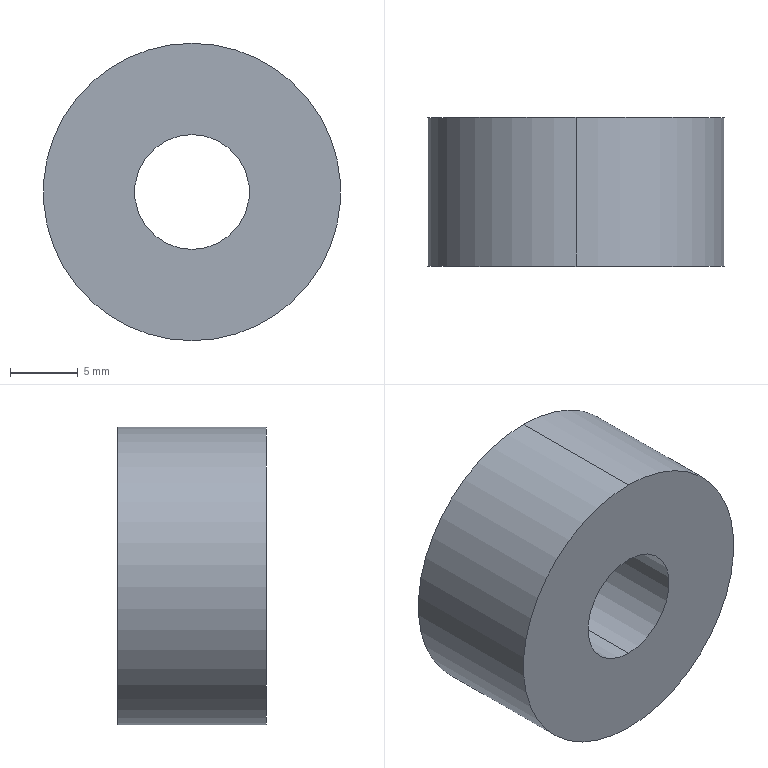Part | SolidWorks | features Extrusion 1, HoleWzd 1 | 1 solid | 6 faces | box 22 x 11 x 22 mm | volume 3557 mm3 | cylinder 4 | plane 2 | commonest cylinder face diameters 8.5 x2 22 x2
STEP:
#1=CARTESIAN_POINT('',(0.,0.,-4.25));
#2=VERTEX_POINT('',#1);
#3=CARTESIAN_POINT('',(0.,0.,4.25));
#4=VERTEX_POINT('',#3);
#5=CARTESIAN_POINT('',(0.,0.,0.));
#6=DIRECTION('',(0.,1.,0.));
#7=DIRECTION('',(0.,0.,1.));
#8=AXIS2_PLACEMENT_3D('',#5,#6,#7);
#9=CIRCLE('',#8,4.25);
#10=EDGE_CURVE('',#2,#4,#9,.T.);
#11=ORIENTED_EDGE('',*,*,#10,.F.);
#12=CARTESIAN_POINT('',(0.,11.,-4.25));
#13=VERTEX_POINT('',#12);
#14=CARTESIAN_POINT('',(0.,11.,-4.25));
#15=DIRECTION('',(0.,1.,0.));
#16=VECTOR('',#15,1000.);
#17=LINE('',#14,#16);
#18=EDGE_CURVE('',#2,#13,#17,.T.);
#19=ORIENTED_EDGE('',*,*,#18,.T.);
#20=CARTESIAN_POINT('',(0.,11.,4.25));
#21=VERTEX_POINT('',#20);
#22=CARTESIAN_POINT('',(0.,11.,0.));
#23=DIRECTION('',(0.,1.,0.));
#24=DIRECTION('',(0.,0.,1.));
#25=AXIS2_PLACEMENT_3D('',#22,#23,#24);
#26=CIRCLE('',#25,4.25);
#27=EDGE_CURVE('',#13,#21,#26,.T.);
#28=ORIENTED_EDGE('',*,*,#27,.T.);
#29=CARTESIAN_POINT('',(0.,11.,4.25));
#30=DIRECTION('',(0.,1.,0.));
#31=VECTOR('',#30,1000.);
#32=LINE('',#29,#31);
#33=EDGE_CURVE('',#4,#21,#32,.T.);
#34=ORIENTED_EDGE('',*,*,#33,.F.);
#35=EDGE_LOOP('',(#11,#19,#28,#34));
#36=FACE_OUTER_BOUND('',#35,.T.);
#37=CARTESIAN_POINT('',(0.,11.,0.));
#38=DIRECTION('',(0.,1.,0.));
#39=DIRECTION('',(0.,0.,1.));
#40=AXIS2_PLACEMENT_3D('',#37,#38,#39);
#41=CYLINDRICAL_SURFACE('',#40,4.25);
#42=ADVANCED_FACE('',(#36),#41,.F.);
#43=CARTESIAN_POINT('',(0.,11.,11.));
#44=VERTEX_POINT('',#43);
#45=CARTESIAN_POINT('',(0.,11.,-11.));
#46=VERTEX_POINT('',#45);
#47=CARTESIAN_POINT('',(0.,11.,0.));
#48=DIRECTION('',(0.,1.,0.));
#49=DIRECTION('',(0.,0.,1.));
#50=AXIS2_PLACEMENT_3D('',#47,#48,#49);
#51=CIRCLE('',#50,11.);
#52=EDGE_CURVE('',#44,#46,#51,.T.);
#53=ORIENTED_EDGE('',*,*,#52,.F.);
#54=CARTESIAN_POINT('',(0.,0.,11.));
#55=VERTEX_POINT('',#54);
#56=CARTESIAN_POINT('',(0.,11.,11.));
#57=DIRECTION('',(0.,-1.,0.));
#58=VECTOR('',#57,1000.);
#59=LINE('',#56,#58);
#60=EDGE_CURVE('',#44,#55,#59,.T.);
#61=ORIENTED_EDGE('',*,*,#60,.T.);
#62=CARTESIAN_POINT('',(0.,0.,-11.));
#63=VERTEX_POINT('',#62);
#64=CARTESIAN_POINT('',(0.,0.,0.));
#65=DIRECTION('',(0.,1.,0.));
#66=DIRECTION('',(0.,0.,1.));
#67=AXIS2_PLACEMENT_3D('',#64,#65,#66);
#68=CIRCLE('',#67,11.);
#69=EDGE_CURVE('',#55,#63,#68,.T.);
#70=ORIENTED_EDGE('',*,*,#69,.T.);
#71=CARTESIAN_POINT('',(0.,11.,-11.));
#72=DIRECTION('',(0.,-1.,0.));
#73=VECTOR('',#72,1000.);
#74=LINE('',#71,#73);
#75=EDGE_CURVE('',#46,#63,#74,.T.);
#76=ORIENTED_EDGE('',*,*,#75,.F.);
#77=EDGE_LOOP('',(#53,#61,#70,#76));
#78=FACE_OUTER_BOUND('',#77,.T.);
#79=CARTESIAN_POINT('',(0.,11.,0.));
#80=DIRECTION('',(0.,-1.,0.));
#81=DIRECTION('',(0.,0.,-1.));
#82=AXIS2_PLACEMENT_3D('',#79,#80,#81);
#83=CYLINDRICAL_SURFACE('',#82,11.);
#84=ADVANCED_FACE('',(#78),#83,.T.);
#85=CARTESIAN_POINT('',(0.,11.,0.));
#86=DIRECTION('',(0.,1.,0.));
#87=DIRECTION('',(0.,0.,1.));
#88=AXIS2_PLACEMENT_3D('',#85,#86,#87);
#89=CIRCLE('',#88,4.25);
#90=EDGE_CURVE('',#21,#13,#89,.T.);
#91=ORIENTED_EDGE('',*,*,#90,.F.);
#92=ORIENTED_EDGE('',*,*,#27,.F.);
#93=EDGE_LOOP('',(#91,#92));
#94=FACE_BOUND('',#93,.T.);
#95=CARTESIAN_POINT('',(0.,11.,0.));
#96=DIRECTION('',(0.,1.,0.));
#97=DIRECTION('',(0.,0.,1.));
#98=AXIS2_PLACEMENT_3D('',#95,#96,#97);
#99=CIRCLE('',#98,11.);
#100=EDGE_CURVE('',#46,#44,#99,.T.);
#101=ORIENTED_EDGE('',*,*,#100,.T.);
#102=ORIENTED_EDGE('',*,*,#52,.T.);
#103=EDGE_LOOP('',(#101,#102));
#104=FACE_OUTER_BOUND('',#103,.T.);
#105=CARTESIAN_POINT('',(0.,11.,0.));
#106=DIRECTION('',(0.,1.,0.));
#107=DIRECTION('',(0.,0.,1.));
#108=AXIS2_PLACEMENT_3D('',#105,#106,#107);
#109=PLANE('',#108);
#110=ADVANCED_FACE('',(#94,#104),#109,.T.);
#111=CARTESIAN_POINT('',(0.,0.,0.));
#112=DIRECTION('',(0.,1.,0.));
#113=DIRECTION('',(0.,0.,1.));
#114=AXIS2_PLACEMENT_3D('',#111,#112,#113);
#115=CIRCLE('',#114,4.25);
#116=EDGE_CURVE('',#4,#2,#115,.T.);
#117=ORIENTED_EDGE('',*,*,#116,.T.);
#118=ORIENTED_EDGE('',*,*,#10,.T.);
#119=EDGE_LOOP('',(#117,#118));
#120=FACE_BOUND('',#119,.T.);
#121=CARTESIAN_POINT('',(0.,0.,0.));
#122=DIRECTION('',(0.,1.,0.));
#123=DIRECTION('',(0.,0.,1.));
#124=AXIS2_PLACEMENT_3D('',#121,#122,#123);
#125=CIRCLE('',#124,11.);
#126=EDGE_CURVE('',#63,#55,#125,.T.);
#127=ORIENTED_EDGE('',*,*,#126,.F.);
#128=ORIENTED_EDGE('',*,*,#69,.F.);
#129=EDGE_LOOP('',(#127,#128));
#130=FACE_OUTER_BOUND('',#129,.T.);
#131=CARTESIAN_POINT('',(0.,0.,0.));
#132=DIRECTION('',(0.,1.,0.));
#133=DIRECTION('',(0.,0.,1.));
#134=AXIS2_PLACEMENT_3D('',#131,#132,#133);
#135=PLANE('',#134);
#136=ADVANCED_FACE('',(#120,#130),#135,.F.);
#137=ORIENTED_EDGE('',*,*,#60,.F.);
#138=ORIENTED_EDGE('',*,*,#100,.F.);
#139=ORIENTED_EDGE('',*,*,#75,.T.);
#140=ORIENTED_EDGE('',*,*,#126,.T.);
#141=EDGE_LOOP('',(#137,#138,#139,#140));
#142=FACE_OUTER_BOUND('',#141,.T.);
#143=CARTESIAN_POINT('',(0.,11.,0.));
#144=DIRECTION('',(0.,-1.,0.));
#145=DIRECTION('',(0.,0.,-1.));
#146=AXIS2_PLACEMENT_3D('',#143,#144,#145);
#147=CYLINDRICAL_SURFACE('',#146,11.);
#148=ADVANCED_FACE('',(#142),#147,.T.);
#149=ORIENTED_EDGE('',*,*,#18,.F.);
#150=ORIENTED_EDGE('',*,*,#116,.F.);
#151=ORIENTED_EDGE('',*,*,#33,.T.);
#152=ORIENTED_EDGE('',*,*,#90,.T.);
#153=EDGE_LOOP('',(#149,#150,#151,#152));
#154=FACE_OUTER_BOUND('',#153,.T.);
#155=CARTESIAN_POINT('',(0.,11.,0.));
#156=DIRECTION('',(0.,1.,0.));
#157=DIRECTION('',(0.,0.,1.));
#158=AXIS2_PLACEMENT_3D('',#155,#156,#157);
#159=CYLINDRICAL_SURFACE('',#158,4.25);
#160=ADVANCED_FACE('',(#154),#159,.F.);
#161=CLOSED_SHELL('',(#42,#84,#110,#136,#148,#160));
#162=MANIFOLD_SOLID_BREP('',#161);
#163=CARTESIAN_POINT('',(0.,0.,0.));
#164=DIRECTION('',(0.,0.,1.));
#165=DIRECTION('',(1.,0.,0.));
#166=AXIS2_PLACEMENT_3D('',#163,#164,#165);
#167=(LENGTH_UNIT()NAMED_UNIT(*)SI_UNIT(.MILLI.,.METRE.));
#168=UNCERTAINTY_MEASURE_WITH_UNIT(LENGTH_MEASURE(0.00001),#167,'','');
#169=(NAMED_UNIT(*)PLANE_ANGLE_UNIT()SI_UNIT($,.RADIAN.));
#170=(NAMED_UNIT(*)SI_UNIT($,.STERADIAN.)SOLID_ANGLE_UNIT());
#171=(GEOMETRIC_REPRESENTATION_CONTEXT(3)GLOBAL_UNCERTAINTY_ASSIGNED_CONTEXT((#168))GLOBAL_UNIT_ASSIGNED_CONTEXT((#167,#169,#170))REPRESENTATION_CONTEXT('',''));
#172=ADVANCED_BREP_SHAPE_REPRESENTATION('',(#162,#166),#171);